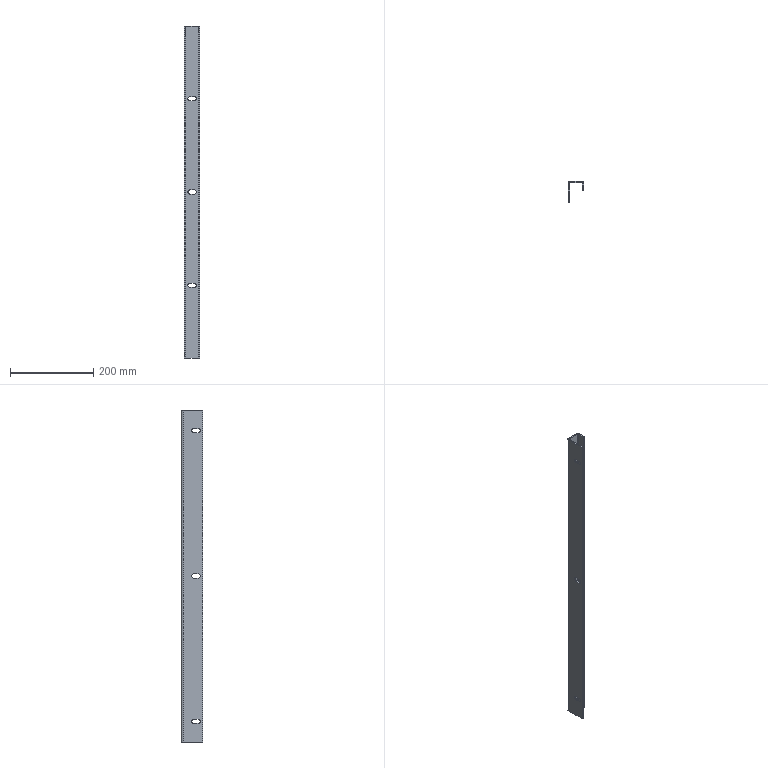Part | SolidWorks | features ICE 3, Cut 1, FlatPattern 1, SMBaseFlange 1, SheetMetal 1 | 1 solid | 57 faces | box 37 x 51 x 800 mm | volume 235979 mm3 | plane 30 | cylinder 27 | commonest cylinder face diameters 10 x9 6 x8 10.5 x6 2 x2 8 x2